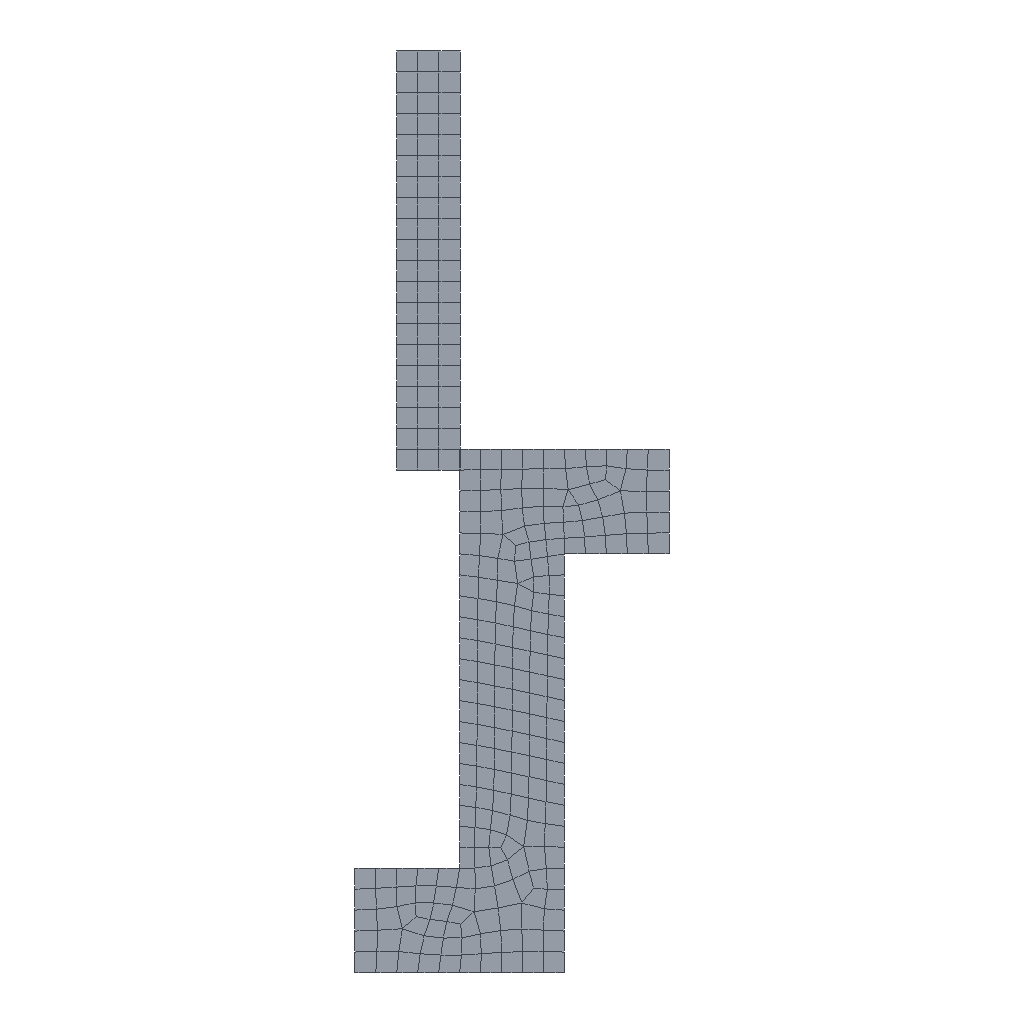Simulation study | abaqus
Set-up summary:
category,name,step,type,value,unit,region
solver,abaqus,,Abaqus/CAE 2024
units,mm-N-s-tonne (MPa),,inferred,E=210000 density=
analysis,Incontact,,static,nlgeom=True; time_period=10
analysis,Press,,static,nlgeom=True; time_period=1
mesh,nodes,,,328
mesh,elements,,,263
element_type,CAX4I,,,261
element_type,CAX3,,,2
material,Material-1,,E,210000
material,Material-1,,nu,0.3
section,Material-1,,solid section,,,_PickedSet2
section,Material-1,,solid section,,,_PickedSet2
bc,BC-Fix-Base,initial,fixed,[dofs=y],,Set-Base-Fix
bc,BC-Move-Punch,Incontact,fixed,"[dofs=rz,x n=2]",,Set-Punch-Ref
bc,BC-Move-Punch,Incontact,displacement,-0.001 [dofs=y],,Set-Punch-Ref
bc,BC-Move-Punch,Press,displacement,-57 [dofs=y],,Set-Punch-Ref
contact,Int-Base-InnerRing,initial,contact pair surface to surface,interaction=IntProp-Friction02; friction=0.2,,Surf-InnerRing-Radial / Surf-Base-Radial
contact,Int-Pro_Friction02,initial,contact pair surface to surface,interaction=IntProp-NoFriction,,Surf-InnerRing-Axial / punch-1.Surf-Punch-Axial
constraint,rigid body,,,1
Abaqus input file, long lists of numbers shortened:
*Heading
** Job name: deck Model name: Model-1
** Generated by: Abaqus/CAE 2024
*Preprint, echo=NO, model=NO, history=NO, contact=NO
**
** PARTS
**
*Part, name=Baes
*Node
      1,          35.,          15.
      2,          35.,           0.
** (241 more lines like these left out)
*Element, type=CAX3
1, 205, 181, 226
2, 214, 149, 157
*Element, type=CAX4I
  3,  85,  11,  12, 241
  4,  11,  85,  84,  10
** (199 more lines like these left out)
*Nset, nset=_PickedSet2, internal, generate
   1,  243,    1
*Elset, elset=_PickedSet2, internal, generate
   1,  203,    1
** Section: Section-1
*Solid Section, elset=_PickedSet2, material=Material-1
,
*End Part
**
*Part, name=InnerRing
*Node
      1,          41.,         132.
      2,          41.,         129.
** (82 more lines like these left out)
*Element, type=CAX4I
 1,  1,  2, 23, 22
 2,  2,  3, 24, 23
** (58 more lines like these left out)
*Nset, nset=_PickedSet2, internal, generate
  1,  84,   1
*Elset, elset=_PickedSet2, internal, generate
  1,  60,   1
** Section: Section-1
*Solid Section, elset=_PickedSet2, material=Material-1
,
*End Part
**
*Part, name=punch
*End Part
**
**
** ASSEMBLY
**
*Assembly, name=Assembly
**
*Instance, name=Baes-1, part=Baes
*End Instance
**
*Instance, name=InnerRing-1, part=InnerRing
*End Instance
**
*Instance, name=punch-1, part=punch
*Node
      1,         45.5,         145.,           0.
*Nset, nset=punch-1-RefPt_, internal
1,
*Surface, type=SEGMENTS, name=Surf-Punch-Axial
START,          56.,         132.
 LINE,          56.,         145.
 LINE,          35.,         145.
 LINE,          35.,         132.
 LINE,          56.,         132.
*Rigid Body, ref node=punch-1-RefPt_, analytical surface=Surf-Punch-Axial
*End Instance
**
*Nset, nset=Set-Base-Fix, instance=Baes-1
  2,  3, 13, 14, 15, 16, 17, 18, 19, 20, 21
*Elset, elset=Set-Base-Fix, instance=Baes-1
  5, 11, 12, 15, 16, 18, 19, 78, 80, 82
*Nset, nset=Set-Punch-Ref, instance=punch-1
 1,
*Elset, elset=_Surf-Base-Radial_S4, internal, instance=Baes-1
  6, 26, 34, 36, 37, 52, 54, 55, 58, 62, 63, 66, 67, 93
*Elset, elset=_Surf-Base-Radial_S2, internal, instance=Baes-1
  51,  94,  97,  98, 100, 102
*Surface, type=ELEMENT, name=Surf-Base-Radial
_Surf-Base-Radial_S4, S4
_Surf-Base-Radial_S2, S2
*Elset, elset=_Surf-InnerRing-Axial_S4, internal, instance=InnerRing-1, generate
  1,  41,  20
*Surface, type=ELEMENT, name=Surf-InnerRing-Axial
_Surf-InnerRing-Axial_S4, S4
*Elset, elset=_Surf-InnerRing-Radial_S3, internal, instance=InnerRing-1, generate
 41,  60,   1
*Surface, type=ELEMENT, name=Surf-InnerRing-Radial
_Surf-InnerRing-Radial_S3, S3
*End Assembly
**
** MATERIALS
**
*Material, name=Material-1
*Elastic
210000., 0.3
**
** INTERACTION PROPERTIES
**
*Surface Interaction, name=IntProp-Friction02
1.,
*Friction, slip tolerance=0.005
 0.2,
*Surface Interaction, name=IntProp-NoFriction
1.,
**
** BOUNDARY CONDITIONS
**
** Name: BC-Fix-Base Type: Displacement/Rotation
*Boundary
Set-Base-Fix, 2, 2
**
** INTERACTIONS
**
** Interaction: Int-Base-InnerRing
*Contact Pair, interaction=IntProp-Friction02, type=SURFACE TO SURFACE
Surf-InnerRing-Radial, Surf-Base-Radial
** Interaction: Int-Pro_Friction02
*Contact Pair, interaction=IntProp-NoFriction, type=SURFACE TO SURFACE
Surf-InnerRing-Axial, punch-1.Surf-Punch-Axial
** ----------------------------------------------------------------
**
** STEP: Incontact
**
*Step, name=Incontact, nlgeom=YES
*Static
0.1, 10., 1e-05, 1.
**
** BOUNDARY CONDITIONS
**
** Name: BC-Move-Punch Type: Displacement/Rotation
*Boundary
Set-Punch-Ref, 1, 1
Set-Punch-Ref, 2, 2, -0.001
Set-Punch-Ref, 6, 6
**
** OUTPUT REQUESTS
**
*Restart, write, frequency=0
*Print, solve=NO
**
** FIELD OUTPUT: F-Output-1
**
*Output, field, variable=PRESELECT
**
** HISTORY OUTPUT: H-Output-1
**
*Output, history
*Contact Output, main=Surf-Base-Radial, secondary=Surf-InnerRing-Radial
CFN1, CFN2, CFN3, CFNM
*End Step
** ----------------------------------------------------------------
**
** STEP: Press
**
*Step, name=Press, nlgeom=YES
*Static
0.05263, 1., 1e-05, 0.05263
**
** BOUNDARY CONDITIONS
**
** Name: BC-Move-Punch Type: Displacement/Rotation
*Boundary
Set-Punch-Ref, 2, 2, -57.
**
** OUTPUT REQUESTS
**
*Restart, write, frequency=0
**
** FIELD OUTPUT: F-Output-1
**
*Output, field, variable=PRESELECT
**
** HISTORY OUTPUT: H-Output-1
**
*Output, history
*Contact Output, main=Surf-Base-Radial, secondary=Surf-InnerRing-Radial
CFN1, CFN2, CFN3, CFNM
*End Step
Results summary:
result,odb.job_status,,,JOB_STATUS_COMPLETED_SUCCESSFULLY,"consistent, unstated (Abaqus has no unit system)"
result,steps[0].procedure,Incontact,,*STATIC,"consistent, unstated (Abaqus has no unit system)"
result,steps[0].time_period,Incontact,,1,"consistent, unstated (Abaqus has no unit system)"
result,steps[0].n_frames,Incontact,,2,"consistent, unstated (Abaqus has no unit system)"
result,steps[0].last_frame.id,Incontact,,1,"consistent, unstated (Abaqus has no unit system)"
result,steps[0].last_frame.value,Incontact,,1,"consistent, unstated (Abaqus has no unit system)"
result,steps[0].last_frame.description,Incontact,,Increment      1: Step Time =    1.000,"consistent, unstated (Abaqus has no unit system)"
result,steps[0].completed,Incontact,,True,"consistent, unstated (Abaqus has no unit system)"
result,steps[0].max_U_magnitude,Incontact,,0.05158,"consistent, unstated (Abaqus has no unit system)"
result,steps[0].max_S_mises,Incontact,,241.55,"consistent, unstated (Abaqus has no unit system)"
result,steps[0].RF_sum[1],Incontact,,0.1003,"consistent, unstated (Abaqus has no unit system)"
result,steps[0].RF_sum[2],Incontact,,-0.007812,"consistent, unstated (Abaqus has no unit system)"
result,steps[0].diagnostic.n_increments,Incontact,,1,"consistent, unstated (Abaqus has no unit system)"
result,steps[1].procedure,Press,,*STATIC,"consistent, unstated (Abaqus has no unit system)"
result,steps[1].time_period,Press,,1,"consistent, unstated (Abaqus has no unit system)"
result,steps[1].n_frames,Press,,21,"consistent, unstated (Abaqus has no unit system)"
result,steps[1].last_frame.id,Press,,20,"consistent, unstated (Abaqus has no unit system)"
result,steps[1].last_frame.value,Press,,1,"consistent, unstated (Abaqus has no unit system)"
result,steps[1].last_frame.description,Press,,Increment     20: Step Time =    1.000,"consistent, unstated (Abaqus has no unit system)"
result,steps[1].completed,Press,,True,"consistent, unstated (Abaqus has no unit system)"
result,steps[1].max_U_magnitude,Press,,57.015,"consistent, unstated (Abaqus has no unit system)"
result,steps[1].max_S_mises,Press,,268.575,"consistent, unstated (Abaqus has no unit system)"
result,steps[1].RF_sum[1],Press,,7.516,"consistent, unstated (Abaqus has no unit system)"
result,steps[1].RF_sum[2],Press,,0.01562,"consistent, unstated (Abaqus has no unit system)"
result,steps[1].diagnostic.n_increments,Press,,20,"consistent, unstated (Abaqus has no unit system)"